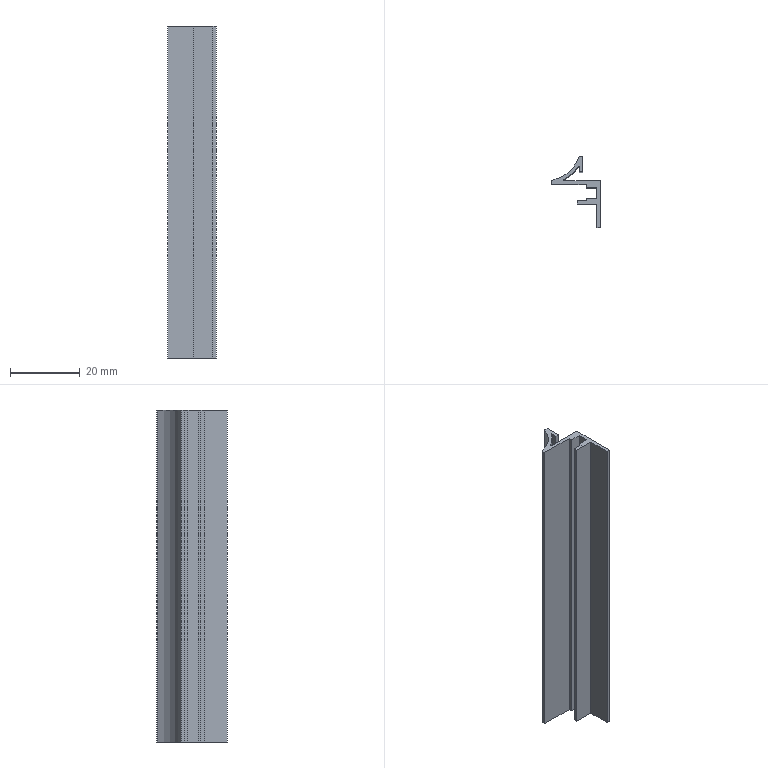Part | SolidWorks | features BaseBody 1, ICE 1, MoveFace 1 | 1 solid | 27 faces | box 14 x 20.3 x 95 mm | volume 4837 mm3 | plane 20 | cylinder 7 | commonest cylinder face diameters 0.387 x2 0.8 x2 0.4 x1 20 x1 22 x1
STEP:
#1=CARTESIAN_POINT('',(-5.304,-0.625,200.));
#2=VERTEX_POINT('',#1);
#3=CARTESIAN_POINT('',(-5.449,-0.8125,200.));
#4=VERTEX_POINT('',#3);
#5=CARTESIAN_POINT('',(-5.255,-0.8125,200.));
#6=DIRECTION('',(0.,0.,1.));
#7=DIRECTION('',(-1.,0.,0.));
#8=AXIS2_PLACEMENT_3D('',#5,#6,#7);
#9=CIRCLE('',#8,0.1937);
#10=EDGE_CURVE('',#2,#4,#9,.T.);
#11=ORIENTED_EDGE('',*,*,#10,.T.);
#12=CARTESIAN_POINT('',(-5.449,-0.8125,105.));
#13=VERTEX_POINT('',#12);
#14=CARTESIAN_POINT('',(-5.449,-0.8125,230.));
#15=DIRECTION('',(0.,0.,-1.));
#16=VECTOR('',#15,1000.);
#17=LINE('',#14,#16);
#18=EDGE_CURVE('',#4,#13,#17,.T.);
#19=ORIENTED_EDGE('',*,*,#18,.T.);
#20=CARTESIAN_POINT('',(-5.304,-0.625,105.));
#21=VERTEX_POINT('',#20);
#22=CARTESIAN_POINT('',(-5.255,-0.8125,105.));
#23=DIRECTION('',(0.,0.,-1.));
#24=DIRECTION('',(1.,0.,0.));
#25=AXIS2_PLACEMENT_3D('',#22,#23,#24);
#26=CIRCLE('',#25,0.1937);
#27=EDGE_CURVE('',#13,#21,#26,.T.);
#28=ORIENTED_EDGE('',*,*,#27,.T.);
#29=CARTESIAN_POINT('',(-5.304,-0.625,230.));
#30=DIRECTION('',(0.,0.,-1.));
#31=VECTOR('',#30,1000.);
#32=LINE('',#29,#31);
#33=EDGE_CURVE('',#2,#21,#32,.T.);
#34=ORIENTED_EDGE('',*,*,#33,.F.);
#35=EDGE_LOOP('',(#11,#19,#28,#34));
#36=FACE_OUTER_BOUND('',#35,.T.);
#37=CARTESIAN_POINT('',(-5.255,-0.8125,230.));
#38=DIRECTION('',(0.,0.,-1.));
#39=DIRECTION('',(-1.,0.,0.));
#40=AXIS2_PLACEMENT_3D('',#37,#38,#39);
#41=CYLINDRICAL_SURFACE('',#40,0.1937);
#42=ADVANCED_FACE('',(#36),#41,.F.);
#43=CARTESIAN_POINT('',(5.,-1.,105.));
#44=VERTEX_POINT('',#43);
#45=CARTESIAN_POINT('',(5.,-14.3,105.));
#46=VERTEX_POINT('',#45);
#47=CARTESIAN_POINT('',(5.,29.623,105.));
#48=DIRECTION('',(0.,-1.,0.));
#49=VECTOR('',#48,1000.);
#50=LINE('',#47,#49);
#51=EDGE_CURVE('',#44,#46,#50,.T.);
#52=ORIENTED_EDGE('',*,*,#51,.F.);
#53=CARTESIAN_POINT('',(5.,-1.,200.));
#54=VERTEX_POINT('',#53);
#55=CARTESIAN_POINT('',(5.,-1.,230.));
#56=DIRECTION('',(0.,0.,-1.));
#57=VECTOR('',#56,1000.);
#58=LINE('',#55,#57);
#59=EDGE_CURVE('',#54,#44,#58,.T.);
#60=ORIENTED_EDGE('',*,*,#59,.F.);
#61=CARTESIAN_POINT('',(5.,-14.3,200.));
#62=VERTEX_POINT('',#61);
#63=CARTESIAN_POINT('',(5.,-14.3,200.));
#64=DIRECTION('',(0.,1.,0.));
#65=VECTOR('',#64,1000.);
#66=LINE('',#63,#65);
#67=EDGE_CURVE('',#62,#54,#66,.T.);
#68=ORIENTED_EDGE('',*,*,#67,.F.);
#69=CARTESIAN_POINT('',(5.,-14.3,230.));
#70=DIRECTION('',(0.,0.,1.));
#71=VECTOR('',#70,1000.);
#72=LINE('',#69,#71);
#73=EDGE_CURVE('',#46,#62,#72,.T.);
#74=ORIENTED_EDGE('',*,*,#73,.F.);
#75=EDGE_LOOP('',(#52,#60,#68,#74));
#76=FACE_OUTER_BOUND('',#75,.T.);
#77=CARTESIAN_POINT('',(5.,-14.3,230.));
#78=DIRECTION('',(-1.,0.,0.));
#79=DIRECTION('',(0.,0.,1.));
#80=AXIS2_PLACEMENT_3D('',#77,#78,#79);
#81=PLANE('',#80);
#82=ADVANCED_FACE('',(#76),#81,.F.);
#83=CARTESIAN_POINT('',(-9.,-2.,105.));
#84=VERTEX_POINT('',#83);
#85=CARTESIAN_POINT('',(-9.,-2.,200.));
#86=VERTEX_POINT('',#85);
#87=CARTESIAN_POINT('',(-9.,-2.,230.));
#88=DIRECTION('',(0.,0.,1.));
#89=VECTOR('',#88,1000.);
#90=LINE('',#87,#89);
#91=EDGE_CURVE('',#84,#86,#90,.T.);
#92=ORIENTED_EDGE('',*,*,#91,.F.);
#93=CARTESIAN_POINT('',(0.9,-2.,105.));
#94=VERTEX_POINT('',#93);
#95=CARTESIAN_POINT('',(5.,-2.,105.));
#96=DIRECTION('',(-1.,0.,0.));
#97=VECTOR('',#96,1000.);
#98=LINE('',#95,#97);
#99=EDGE_CURVE('',#94,#84,#98,.T.);
#100=ORIENTED_EDGE('',*,*,#99,.F.);
#101=CARTESIAN_POINT('',(0.9,-2.,200.));
#102=VERTEX_POINT('',#101);
#103=CARTESIAN_POINT('',(0.9,-2.,230.));
#104=DIRECTION('',(0.,0.,-1.));
#105=VECTOR('',#104,1000.);
#106=LINE('',#103,#105);
#107=EDGE_CURVE('',#102,#94,#106,.T.);
#108=ORIENTED_EDGE('',*,*,#107,.F.);
#109=CARTESIAN_POINT('',(5.,-2.,200.));
#110=DIRECTION('',(1.,0.,0.));
#111=VECTOR('',#110,1000.);
#112=LINE('',#109,#111);
#113=EDGE_CURVE('',#86,#102,#112,.T.);
#114=ORIENTED_EDGE('',*,*,#113,.F.);
#115=EDGE_LOOP('',(#92,#100,#108,#114));
#116=FACE_OUTER_BOUND('',#115,.T.);
#117=CARTESIAN_POINT('',(-9.,-2.,230.));
#118=DIRECTION('',(0.,1.,0.));
#119=DIRECTION('',(0.,0.,1.));
#120=AXIS2_PLACEMENT_3D('',#117,#118,#119);
#121=PLANE('',#120);
#122=ADVANCED_FACE('',(#116),#121,.F.);
#123=CARTESIAN_POINT('',(4.,-6.,200.));
#124=VERTEX_POINT('',#123);
#125=CARTESIAN_POINT('',(4.,-3.,200.));
#126=VERTEX_POINT('',#125);
#127=CARTESIAN_POINT('',(4.,29.623,200.));
#128=DIRECTION('',(0.,1.,0.));
#129=VECTOR('',#128,1000.);
#130=LINE('',#127,#129);
#131=EDGE_CURVE('',#124,#126,#130,.T.);
#132=ORIENTED_EDGE('',*,*,#131,.F.);
#133=CARTESIAN_POINT('',(1.,-6.,200.));
#134=VERTEX_POINT('',#133);
#135=CARTESIAN_POINT('',(5.,-6.,200.));
#136=DIRECTION('',(1.,0.,0.));
#137=VECTOR('',#136,1000.);
#138=LINE('',#135,#137);
#139=EDGE_CURVE('',#134,#124,#138,.T.);
#140=ORIENTED_EDGE('',*,*,#139,.F.);
#141=CARTESIAN_POINT('',(1.,-6.7,200.));
#142=VERTEX_POINT('',#141);
#143=CARTESIAN_POINT('',(1.,-6.,200.));
#144=DIRECTION('',(0.,-1.,0.));
#145=VECTOR('',#144,1000.);
#146=LINE('',#143,#145);
#147=EDGE_CURVE('',#134,#142,#146,.T.);
#148=ORIENTED_EDGE('',*,*,#147,.T.);
#149=CARTESIAN_POINT('',(-1.7,-6.7,200.));
#150=VERTEX_POINT('',#149);
#151=CARTESIAN_POINT('',(5.,-6.7,200.));
#152=DIRECTION('',(1.,0.,0.));
#153=VECTOR('',#152,1000.);
#154=LINE('',#151,#153);
#155=EDGE_CURVE('',#150,#142,#154,.T.);
#156=ORIENTED_EDGE('',*,*,#155,.F.);
#157=CARTESIAN_POINT('',(-1.7,-7.7,200.));
#158=VERTEX_POINT('',#157);
#159=CARTESIAN_POINT('',(-1.7,-6.7,200.));
#160=DIRECTION('',(0.,-1.,0.));
#161=VECTOR('',#160,1000.);
#162=LINE('',#159,#161);
#163=EDGE_CURVE('',#150,#158,#162,.T.);
#164=ORIENTED_EDGE('',*,*,#163,.T.);
#165=CARTESIAN_POINT('',(4.,-7.7,200.));
#166=VERTEX_POINT('',#165);
#167=CARTESIAN_POINT('',(5.,-7.7,200.));
#168=DIRECTION('',(-1.,0.,0.));
#169=VECTOR('',#168,1000.);
#170=LINE('',#167,#169);
#171=EDGE_CURVE('',#166,#158,#170,.T.);
#172=ORIENTED_EDGE('',*,*,#171,.F.);
#173=CARTESIAN_POINT('',(4.,-14.3,200.));
#174=VERTEX_POINT('',#173);
#175=CARTESIAN_POINT('',(4.,29.623,200.));
#176=DIRECTION('',(0.,1.,0.));
#177=VECTOR('',#176,1000.);
#178=LINE('',#175,#177);
#179=EDGE_CURVE('',#174,#166,#178,.T.);
#180=ORIENTED_EDGE('',*,*,#179,.F.);
#181=CARTESIAN_POINT('',(5.,-14.3,200.));
#182=DIRECTION('',(-1.,0.,0.));
#183=VECTOR('',#182,1000.);
#184=LINE('',#181,#183);
#185=EDGE_CURVE('',#62,#174,#184,.T.);
#186=ORIENTED_EDGE('',*,*,#185,.F.);
#187=ORIENTED_EDGE('',*,*,#67,.T.);
#188=CARTESIAN_POINT('',(-5.207,-1.,200.));
#189=VERTEX_POINT('',#188);
#190=CARTESIAN_POINT('',(5.,-1.,200.));
#191=DIRECTION('',(1.,0.,0.));
#192=VECTOR('',#191,1000.);
#193=LINE('',#190,#192);
#194=EDGE_CURVE('',#189,#54,#193,.T.);
#195=ORIENTED_EDGE('',*,*,#194,.F.);
#196=CARTESIAN_POINT('',(-5.255,-0.8125,200.));
#197=DIRECTION('',(0.,0.,1.));
#198=DIRECTION('',(-1.,0.,0.));
#199=AXIS2_PLACEMENT_3D('',#196,#197,#198);
#200=CIRCLE('',#199,0.1937);
#201=EDGE_CURVE('',#4,#189,#200,.T.);
#202=ORIENTED_EDGE('',*,*,#201,.F.);
#203=ORIENTED_EDGE('',*,*,#10,.F.);
#204=CARTESIAN_POINT('',(-1.368,3.063,200.));
#205=VERTEX_POINT('',#204);
#206=CARTESIAN_POINT('',(-10.628,9.,200.));
#207=DIRECTION('',(0.,0.,1.));
#208=DIRECTION('',(-1.,0.,0.));
#209=AXIS2_PLACEMENT_3D('',#206,#207,#208);
#210=CIRCLE('',#209,11.);
#211=EDGE_CURVE('',#2,#205,#210,.T.);
#212=ORIENTED_EDGE('',*,*,#211,.T.);
#213=CARTESIAN_POINT('',(-1.,2.955,200.));
#214=VERTEX_POINT('',#213);
#215=CARTESIAN_POINT('',(-1.2,2.955,200.));
#216=DIRECTION('',(0.,0.,1.));
#217=DIRECTION('',(-1.,0.,0.));
#218=AXIS2_PLACEMENT_3D('',#215,#216,#217);
#219=CIRCLE('',#218,0.2);
#220=EDGE_CURVE('',#214,#205,#219,.T.);
#221=ORIENTED_EDGE('',*,*,#220,.F.);
#222=CARTESIAN_POINT('',(-1.,1.5,200.));
#223=VERTEX_POINT('',#222);
#224=CARTESIAN_POINT('',(-1.,2.955,200.));
#225=DIRECTION('',(0.,1.,0.));
#226=VECTOR('',#225,1000.);
#227=LINE('',#224,#226);
#228=EDGE_CURVE('',#223,#214,#227,.T.);
#229=ORIENTED_EDGE('',*,*,#228,.F.);
#230=CARTESIAN_POINT('',(0.,1.5,200.));
#231=VERTEX_POINT('',#230);
#232=CARTESIAN_POINT('',(-1.,1.5,200.));
#233=DIRECTION('',(-1.,0.,0.));
#234=VECTOR('',#233,1000.);
#235=LINE('',#232,#234);
#236=EDGE_CURVE('',#231,#223,#235,.T.);
#237=ORIENTED_EDGE('',*,*,#236,.F.);
#238=CARTESIAN_POINT('',(0.,6.,200.));
#239=VERTEX_POINT('',#238);
#240=CARTESIAN_POINT('',(0.,1.5,200.));
#241=DIRECTION('',(0.,-1.,0.));
#242=VECTOR('',#241,1000.);
#243=LINE('',#240,#242);
#244=EDGE_CURVE('',#239,#231,#243,.T.);
#245=ORIENTED_EDGE('',*,*,#244,.F.);
#246=CARTESIAN_POINT('',(-0.8,6.,200.));
#247=VERTEX_POINT('',#246);
#248=CARTESIAN_POINT('',(0.,6.,200.));
#249=DIRECTION('',(1.,0.,0.));
#250=VECTOR('',#249,1000.);
#251=LINE('',#248,#250);
#252=EDGE_CURVE('',#247,#239,#251,.T.);
#253=ORIENTED_EDGE('',*,*,#252,.F.);
#254=CARTESIAN_POINT('',(-1.178,5.731,200.));
#255=VERTEX_POINT('',#254);
#256=CARTESIAN_POINT('',(-0.8,5.6,200.));
#257=DIRECTION('',(0.,0.,1.));
#258=DIRECTION('',(-1.,0.,0.));
#259=AXIS2_PLACEMENT_3D('',#256,#257,#258);
#260=CIRCLE('',#259,0.4);
#261=EDGE_CURVE('',#247,#255,#260,.T.);
#262=ORIENTED_EDGE('',*,*,#261,.T.);
#263=CARTESIAN_POINT('',(-8.678,-0.8077,200.));
#264=VERTEX_POINT('',#263);
#265=CARTESIAN_POINT('',(-10.628,9.,200.));
#266=DIRECTION('',(0.,0.,1.));
#267=DIRECTION('',(-1.,0.,0.));
#268=AXIS2_PLACEMENT_3D('',#265,#266,#267);
#269=CIRCLE('',#268,10.);
#270=EDGE_CURVE('',#264,#255,#269,.T.);
#271=ORIENTED_EDGE('',*,*,#270,.F.);
#272=CARTESIAN_POINT('',(-9.,-1.2,200.));
#273=VERTEX_POINT('',#272);
#274=CARTESIAN_POINT('',(-8.6,-1.2,200.));
#275=DIRECTION('',(0.,0.,1.));
#276=DIRECTION('',(-1.,0.,0.));
#277=AXIS2_PLACEMENT_3D('',#274,#275,#276);
#278=CIRCLE('',#277,0.4);
#279=EDGE_CURVE('',#264,#273,#278,.T.);
#280=ORIENTED_EDGE('',*,*,#279,.T.);
#281=CARTESIAN_POINT('',(-9.,8.,200.));
#282=DIRECTION('',(0.,-1.,0.));
#283=VECTOR('',#282,1000.);
#284=LINE('',#281,#283);
#285=EDGE_CURVE('',#273,#86,#284,.T.);
#286=ORIENTED_EDGE('',*,*,#285,.T.);
#287=ORIENTED_EDGE('',*,*,#113,.T.);
#288=CARTESIAN_POINT('',(0.9,-3.,200.));
#289=VERTEX_POINT('',#288);
#290=CARTESIAN_POINT('',(0.9,29.623,200.));
#291=DIRECTION('',(0.,1.,0.));
#292=VECTOR('',#291,1000.);
#293=LINE('',#290,#292);
#294=EDGE_CURVE('',#289,#102,#293,.T.);
#295=ORIENTED_EDGE('',*,*,#294,.F.);
#296=CARTESIAN_POINT('',(5.,-3.,200.));
#297=DIRECTION('',(-1.,0.,0.));
#298=VECTOR('',#297,1000.);
#299=LINE('',#296,#298);
#300=EDGE_CURVE('',#126,#289,#299,.T.);
#301=ORIENTED_EDGE('',*,*,#300,.F.);
#302=EDGE_LOOP('',(#132,#140,#148,#156,#164,#172,#180,#186,#187,#195,#202,#203,#212,#221,#229,#237,#245,#253,#262,#271,#280,#286,#287,#295,#301));
#303=FACE_OUTER_BOUND('',#302,.T.);
#304=CARTESIAN_POINT('',(5.,29.623,200.));
#305=DIRECTION('',(0.,0.,-1.));
#306=DIRECTION('',(-1.,0.,0.));
#307=AXIS2_PLACEMENT_3D('',#304,#305,#306);
#308=PLANE('',#307);
#309=ADVANCED_FACE('',(#303),#308,.F.);
#310=ORIENTED_EDGE('',*,*,#185,.T.);
#311=CARTESIAN_POINT('',(4.,-14.3,105.));
#312=VERTEX_POINT('',#311);
#313=CARTESIAN_POINT('',(4.,-14.3,230.));
#314=DIRECTION('',(0.,0.,1.));
#315=VECTOR('',#314,1000.);
#316=LINE('',#313,#315);
#317=EDGE_CURVE('',#312,#174,#316,.T.);
#318=ORIENTED_EDGE('',*,*,#317,.F.);
#319=CARTESIAN_POINT('',(5.,-14.3,105.));
#320=DIRECTION('',(-1.,0.,0.));
#321=VECTOR('',#320,1000.);
#322=LINE('',#319,#321);
#323=EDGE_CURVE('',#46,#312,#322,.T.);
#324=ORIENTED_EDGE('',*,*,#323,.F.);
#325=ORIENTED_EDGE('',*,*,#73,.T.);
#326=EDGE_LOOP('',(#310,#318,#324,#325));
#327=FACE_OUTER_BOUND('',#326,.T.);
#328=CARTESIAN_POINT('',(4.,-14.3,230.));
#329=DIRECTION('',(0.,1.,0.));
#330=DIRECTION('',(0.,0.,1.));
#331=AXIS2_PLACEMENT_3D('',#328,#329,#330);
#332=PLANE('',#331);
#333=ADVANCED_FACE('',(#327),#332,.F.);
#334=ORIENTED_EDGE('',*,*,#51,.T.);
#335=ORIENTED_EDGE('',*,*,#323,.T.);
#336=CARTESIAN_POINT('',(4.,-7.7,105.));
#337=VERTEX_POINT('',#336);
#338=CARTESIAN_POINT('',(4.,-7.7,105.));
#339=DIRECTION('',(0.,-1.,0.));
#340=VECTOR('',#339,1000.);
#341=LINE('',#338,#340);
#342=EDGE_CURVE('',#337,#312,#341,.T.);
#343=ORIENTED_EDGE('',*,*,#342,.F.);
#344=CARTESIAN_POINT('',(-1.7,-7.7,105.));
#345=VERTEX_POINT('',#344);
#346=CARTESIAN_POINT('',(-1.7,-7.7,105.));
#347=DIRECTION('',(1.,0.,0.));
#348=VECTOR('',#347,1000.);
#349=LINE('',#346,#348);
#350=EDGE_CURVE('',#345,#337,#349,.T.);
#351=ORIENTED_EDGE('',*,*,#350,.F.);
#352=CARTESIAN_POINT('',(-1.7,-6.7,105.));
#353=VERTEX_POINT('',#352);
#354=CARTESIAN_POINT('',(-1.7,29.623,105.));
#355=DIRECTION('',(0.,1.,0.));
#356=VECTOR('',#355,1000.);
#357=LINE('',#354,#356);
#358=EDGE_CURVE('',#345,#353,#357,.T.);
#359=ORIENTED_EDGE('',*,*,#358,.T.);
#360=CARTESIAN_POINT('',(1.,-6.7,105.));
#361=VERTEX_POINT('',#360);
#362=CARTESIAN_POINT('',(1.,-6.7,105.));
#363=DIRECTION('',(-1.,0.,0.));
#364=VECTOR('',#363,1000.);
#365=LINE('',#362,#364);
#366=EDGE_CURVE('',#361,#353,#365,.T.);
#367=ORIENTED_EDGE('',*,*,#366,.F.);
#368=CARTESIAN_POINT('',(1.,-6.,105.));
#369=VERTEX_POINT('',#368);
#370=CARTESIAN_POINT('',(1.,29.623,105.));
#371=DIRECTION('',(0.,1.,0.));
#372=VECTOR('',#371,1000.);
#373=LINE('',#370,#372);
#374=EDGE_CURVE('',#361,#369,#373,.T.);
#375=ORIENTED_EDGE('',*,*,#374,.T.);
#376=CARTESIAN_POINT('',(4.,-6.,105.));
#377=VERTEX_POINT('',#376);
#378=CARTESIAN_POINT('',(4.,-6.,105.));
#379=DIRECTION('',(-1.,0.,0.));
#380=VECTOR('',#379,1000.);
#381=LINE('',#378,#380);
#382=EDGE_CURVE('',#377,#369,#381,.T.);
#383=ORIENTED_EDGE('',*,*,#382,.F.);
#384=CARTESIAN_POINT('',(4.,-3.,105.));
#385=VERTEX_POINT('',#384);
#386=CARTESIAN_POINT('',(4.,-3.,105.));
#387=DIRECTION('',(0.,-1.,0.));
#388=VECTOR('',#387,1000.);
#389=LINE('',#386,#388);
#390=EDGE_CURVE('',#385,#377,#389,.T.);
#391=ORIENTED_EDGE('',*,*,#390,.F.);
#392=CARTESIAN_POINT('',(0.9,-3.,105.));
#393=VERTEX_POINT('',#392);
#394=CARTESIAN_POINT('',(0.9,-3.,105.));
#395=DIRECTION('',(1.,0.,0.));
#396=VECTOR('',#395,1000.);
#397=LINE('',#394,#396);
#398=EDGE_CURVE('',#393,#385,#397,.T.);
#399=ORIENTED_EDGE('',*,*,#398,.F.);
#400=CARTESIAN_POINT('',(0.9,-2.,105.));
#401=DIRECTION('',(0.,-1.,0.));
#402=VECTOR('',#401,1000.);
#403=LINE('',#400,#402);
#404=EDGE_CURVE('',#94,#393,#403,.T.);
#405=ORIENTED_EDGE('',*,*,#404,.F.);
#406=ORIENTED_EDGE('',*,*,#99,.T.);
#407=CARTESIAN_POINT('',(-9.,-1.2,105.));
#408=VERTEX_POINT('',#407);
#409=CARTESIAN_POINT('',(-9.,-1.2,105.));
#410=DIRECTION('',(0.,-1.,0.));
#411=VECTOR('',#410,1000.);
#412=LINE('',#409,#411);
#413=EDGE_CURVE('',#408,#84,#412,.T.);
#414=ORIENTED_EDGE('',*,*,#413,.F.);
#415=CARTESIAN_POINT('',(-8.678,-0.8077,105.));
#416=VERTEX_POINT('',#415);
#417=CARTESIAN_POINT('',(-8.6,-1.2,105.));
#418=DIRECTION('',(0.,0.,-1.));
#419=DIRECTION('',(1.,0.,0.));
#420=AXIS2_PLACEMENT_3D('',#417,#418,#419);
#421=CIRCLE('',#420,0.4);
#422=EDGE_CURVE('',#408,#416,#421,.T.);
#423=ORIENTED_EDGE('',*,*,#422,.T.);
#424=CARTESIAN_POINT('',(-1.178,5.731,105.));
#425=VERTEX_POINT('',#424);
#426=CARTESIAN_POINT('',(-10.628,9.,105.));
#427=DIRECTION('',(0.,0.,-1.));
#428=DIRECTION('',(1.,0.,0.));
#429=AXIS2_PLACEMENT_3D('',#426,#427,#428);
#430=CIRCLE('',#429,10.);
#431=EDGE_CURVE('',#425,#416,#430,.T.);
#432=ORIENTED_EDGE('',*,*,#431,.F.);
#433=CARTESIAN_POINT('',(-0.8,6.,105.));
#434=VERTEX_POINT('',#433);
#435=CARTESIAN_POINT('',(-0.8,5.6,105.));
#436=DIRECTION('',(0.,0.,-1.));
#437=DIRECTION('',(1.,0.,0.));
#438=AXIS2_PLACEMENT_3D('',#435,#436,#437);
#439=CIRCLE('',#438,0.4);
#440=EDGE_CURVE('',#425,#434,#439,.T.);
#441=ORIENTED_EDGE('',*,*,#440,.T.);
#442=CARTESIAN_POINT('',(0.,6.,105.));
#443=VERTEX_POINT('',#442);
#444=CARTESIAN_POINT('',(0.,6.,105.));
#445=DIRECTION('',(-1.,0.,0.));
#446=VECTOR('',#445,1000.);
#447=LINE('',#444,#446);
#448=EDGE_CURVE('',#443,#434,#447,.T.);
#449=ORIENTED_EDGE('',*,*,#448,.F.);
#450=CARTESIAN_POINT('',(0.,1.5,105.));
#451=VERTEX_POINT('',#450);
#452=CARTESIAN_POINT('',(0.,1.5,105.));
#453=DIRECTION('',(0.,1.,0.));
#454=VECTOR('',#453,1000.);
#455=LINE('',#452,#454);
#456=EDGE_CURVE('',#451,#443,#455,.T.);
#457=ORIENTED_EDGE('',*,*,#456,.F.);
#458=CARTESIAN_POINT('',(-1.,1.5,105.));
#459=VERTEX_POINT('',#458);
#460=CARTESIAN_POINT('',(-1.,1.5,105.));
#461=DIRECTION('',(1.,0.,0.));
#462=VECTOR('',#461,1000.);
#463=LINE('',#460,#462);
#464=EDGE_CURVE('',#459,#451,#463,.T.);
#465=ORIENTED_EDGE('',*,*,#464,.F.);
#466=CARTESIAN_POINT('',(-1.,2.955,105.));
#467=VERTEX_POINT('',#466);
#468=CARTESIAN_POINT('',(-1.,2.955,105.));
#469=DIRECTION('',(0.,-1.,0.));
#470=VECTOR('',#469,1000.);
#471=LINE('',#468,#470);
#472=EDGE_CURVE('',#467,#459,#471,.T.);
#473=ORIENTED_EDGE('',*,*,#472,.F.);
#474=CARTESIAN_POINT('',(-1.368,3.063,105.));
#475=VERTEX_POINT('',#474);
#476=CARTESIAN_POINT('',(-1.2,2.955,105.));
#477=DIRECTION('',(0.,0.,-1.));
#478=DIRECTION('',(1.,0.,0.));
#479=AXIS2_PLACEMENT_3D('',#476,#477,#478);
#480=CIRCLE('',#479,0.2);
#481=EDGE_CURVE('',#475,#467,#480,.T.);
#482=ORIENTED_EDGE('',*,*,#481,.F.);
#483=CARTESIAN_POINT('',(-10.628,9.,105.));
#484=DIRECTION('',(0.,0.,-1.));
#485=DIRECTION('',(1.,0.,0.));
#486=AXIS2_PLACEMENT_3D('',#483,#484,#485);
#487=CIRCLE('',#486,11.);
#488=EDGE_CURVE('',#475,#21,#487,.T.);
#489=ORIENTED_EDGE('',*,*,#488,.T.);
#490=ORIENTED_EDGE('',*,*,#27,.F.);
#491=CARTESIAN_POINT('',(-5.207,-1.,105.));
#492=VERTEX_POINT('',#491);
#493=CARTESIAN_POINT('',(-5.255,-0.8125,105.));
#494=DIRECTION('',(0.,0.,-1.));
#495=DIRECTION('',(1.,0.,0.));
#496=AXIS2_PLACEMENT_3D('',#493,#494,#495);
#497=CIRCLE('',#496,0.1937);
#498=EDGE_CURVE('',#492,#13,#497,.T.);
#499=ORIENTED_EDGE('',*,*,#498,.F.);
#500=CARTESIAN_POINT('',(5.,-1.,105.));
#501=DIRECTION('',(-1.,0.,0.));
#502=VECTOR('',#501,1000.);
#503=LINE('',#500,#502);
#504=EDGE_CURVE('',#44,#492,#503,.T.);
#505=ORIENTED_EDGE('',*,*,#504,.F.);
#506=EDGE_LOOP('',(#334,#335,#343,#351,#359,#367,#375,#383,#391,#399,#405,#406,#414,#423,#432,#441,#449,#457,#465,#473,#482,#489,#490,#499,#505));
#507=FACE_OUTER_BOUND('',#506,.T.);
#508=CARTESIAN_POINT('',(5.,29.623,105.));
#509=DIRECTION('',(0.,0.,1.));
#510=DIRECTION('',(1.,0.,0.));
#511=AXIS2_PLACEMENT_3D('',#508,#509,#510);
#512=PLANE('',#511);
#513=ADVANCED_FACE('',(#507),#512,.F.);
#514=ORIENTED_EDGE('',*,*,#59,.T.);
#515=ORIENTED_EDGE('',*,*,#504,.T.);
#516=CARTESIAN_POINT('',(-5.207,-1.,230.));
#517=DIRECTION('',(0.,0.,-1.));
#518=VECTOR('',#517,1000.);
#519=LINE('',#516,#518);
#520=EDGE_CURVE('',#189,#492,#519,.T.);
#521=ORIENTED_EDGE('',*,*,#520,.F.);
#522=ORIENTED_EDGE('',*,*,#194,.T.);
#523=EDGE_LOOP('',(#514,#515,#521,#522));
#524=FACE_OUTER_BOUND('',#523,.T.);
#525=CARTESIAN_POINT('',(5.,-1.,230.));
#526=DIRECTION('',(0.,-1.,0.));
#527=DIRECTION('',(0.,0.,-1.));
#528=AXIS2_PLACEMENT_3D('',#525,#526,#527);
#529=PLANE('',#528);
#530=ADVANCED_FACE('',(#524),#529,.F.);
#531=CARTESIAN_POINT('',(-9.,-1.2,230.));
#532=DIRECTION('',(0.,0.,1.));
#533=VECTOR('',#532,1000.);
#534=LINE('',#531,#533);
#535=EDGE_CURVE('',#408,#273,#534,.T.);
#536=ORIENTED_EDGE('',*,*,#535,.F.);
#537=ORIENTED_EDGE('',*,*,#413,.T.);
#538=ORIENTED_EDGE('',*,*,#91,.T.);
#539=ORIENTED_EDGE('',*,*,#285,.F.);
#540=EDGE_LOOP('',(#536,#537,#538,#539));
#541=FACE_OUTER_BOUND('',#540,.T.);
#542=CARTESIAN_POINT('',(-9.,-1.2,230.));
#543=DIRECTION('',(1.,0.,0.));
#544=DIRECTION('',(0.,0.,-1.));
#545=AXIS2_PLACEMENT_3D('',#542,#543,#544);
#546=PLANE('',#545);
#547=ADVANCED_FACE('',(#541),#546,.F.);
#548=ORIENTED_EDGE('',*,*,#294,.T.);
#549=ORIENTED_EDGE('',*,*,#107,.T.);
#550=ORIENTED_EDGE('',*,*,#404,.T.);
#551=CARTESIAN_POINT('',(0.9,-3.,230.));
#552=DIRECTION('',(0.,0.,-1.));
#553=VECTOR('',#552,1000.);
#554=LINE('',#551,#553);
#555=EDGE_CURVE('',#289,#393,#554,.T.);
#556=ORIENTED_EDGE('',*,*,#555,.F.);
#557=EDGE_LOOP('',(#548,#549,#550,#556));
#558=FACE_OUTER_BOUND('',#557,.T.);
#559=CARTESIAN_POINT('',(0.9,-2.,230.));
#560=DIRECTION('',(1.,0.,0.));
#561=DIRECTION('',(0.,0.,-1.));
#562=AXIS2_PLACEMENT_3D('',#559,#560,#561);
#563=PLANE('',#562);
#564=ADVANCED_FACE('',(#558),#563,.F.);
#565=ORIENTED_EDGE('',*,*,#300,.T.);
#566=ORIENTED_EDGE('',*,*,#555,.T.);
#567=ORIENTED_EDGE('',*,*,#398,.T.);
#568=CARTESIAN_POINT('',(4.,-3.,230.));
#569=DIRECTION('',(0.,0.,-1.));
#570=VECTOR('',#569,1000.);
#571=LINE('',#568,#570);
#572=EDGE_CURVE('',#126,#385,#571,.T.);
#573=ORIENTED_EDGE('',*,*,#572,.F.);
#574=EDGE_LOOP('',(#565,#566,#567,#573));
#575=FACE_OUTER_BOUND('',#574,.T.);
#576=CARTESIAN_POINT('',(0.9,-3.,230.));
#577=DIRECTION('',(0.,1.,0.));
#578=DIRECTION('',(0.,0.,1.));
#579=AXIS2_PLACEMENT_3D('',#576,#577,#578);
#580=PLANE('',#579);
#581=ADVANCED_FACE('',(#575),#580,.F.);
#582=ORIENTED_EDGE('',*,*,#131,.T.);
#583=ORIENTED_EDGE('',*,*,#572,.T.);
#584=ORIENTED_EDGE('',*,*,#390,.T.);
#585=CARTESIAN_POINT('',(4.,-6.,230.));
#586=DIRECTION('',(0.,0.,-1.));
#587=VECTOR('',#586,1000.);
#588=LINE('',#585,#587);
#589=EDGE_CURVE('',#124,#377,#588,.T.);
#590=ORIENTED_EDGE('',*,*,#589,.F.);
#591=EDGE_LOOP('',(#582,#583,#584,#590));
#592=FACE_OUTER_BOUND('',#591,.T.);
#593=CARTESIAN_POINT('',(4.,-3.,230.));
#594=DIRECTION('',(1.,0.,0.));
#595=DIRECTION('',(0.,0.,-1.));
#596=AXIS2_PLACEMENT_3D('',#593,#594,#595);
#597=PLANE('',#596);
#598=ADVANCED_FACE('',(#592),#597,.F.);
#599=ORIENTED_EDGE('',*,*,#139,.T.);
#600=ORIENTED_EDGE('',*,*,#589,.T.);
#601=ORIENTED_EDGE('',*,*,#382,.T.);
#602=CARTESIAN_POINT('',(1.,-6.,230.));
#603=DIRECTION('',(0.,0.,-1.));
#604=VECTOR('',#603,1000.);
#605=LINE('',#602,#604);
#606=EDGE_CURVE('',#134,#369,#605,.T.);
#607=ORIENTED_EDGE('',*,*,#606,.F.);
#608=EDGE_LOOP('',(#599,#600,#601,#607));
#609=FACE_OUTER_BOUND('',#608,.T.);
#610=CARTESIAN_POINT('',(4.,-6.,230.));
#611=DIRECTION('',(0.,-1.,0.));
#612=DIRECTION('',(0.,0.,-1.));
#613=AXIS2_PLACEMENT_3D('',#610,#611,#612);
#614=PLANE('',#613);
#615=ADVANCED_FACE('',(#609),#614,.F.);
#616=ORIENTED_EDGE('',*,*,#155,.T.);
#617=CARTESIAN_POINT('',(1.,-6.7,230.));
#618=DIRECTION('',(0.,0.,1.));
#619=VECTOR('',#618,1000.);
#620=LINE('',#617,#619);
#621=EDGE_CURVE('',#361,#142,#620,.T.);
#622=ORIENTED_EDGE('',*,*,#621,.F.);
#623=ORIENTED_EDGE('',*,*,#366,.T.);
#624=CARTESIAN_POINT('',(-1.7,-6.7,230.));
#625=DIRECTION('',(0.,0.,-1.));
#626=VECTOR('',#625,1000.);
#627=LINE('',#624,#626);
#628=EDGE_CURVE('',#150,#353,#627,.T.);
#629=ORIENTED_EDGE('',*,*,#628,.F.);
#630=EDGE_LOOP('',(#616,#622,#623,#629));
#631=FACE_OUTER_BOUND('',#630,.T.);
#632=CARTESIAN_POINT('',(1.,-6.7,230.));
#633=DIRECTION('',(0.,-1.,0.));
#634=DIRECTION('',(0.,0.,-1.));
#635=AXIS2_PLACEMENT_3D('',#632,#633,#634);
#636=PLANE('',#635);
#637=ADVANCED_FACE('',(#631),#636,.F.);
#638=ORIENTED_EDGE('',*,*,#171,.T.);
#639=CARTESIAN_POINT('',(-1.7,-7.7,230.));
#640=DIRECTION('',(0.,0.,1.));
#641=VECTOR('',#640,1000.);
#642=LINE('',#639,#641);
#643=EDGE_CURVE('',#345,#158,#642,.T.);
#644=ORIENTED_EDGE('',*,*,#643,.F.);
#645=ORIENTED_EDGE('',*,*,#350,.T.);
#646=CARTESIAN_POINT('',(4.,-7.7,230.));
#647=DIRECTION('',(0.,0.,-1.));
#648=VECTOR('',#647,1000.);
#649=LINE('',#646,#648);
#650=EDGE_CURVE('',#166,#337,#649,.T.);
#651=ORIENTED_EDGE('',*,*,#650,.F.);
#652=EDGE_LOOP('',(#638,#644,#645,#651));
#653=FACE_OUTER_BOUND('',#652,.T.);
#654=CARTESIAN_POINT('',(-1.7,-7.7,230.));
#655=DIRECTION('',(0.,1.,0.));
#656=DIRECTION('',(0.,0.,1.));
#657=AXIS2_PLACEMENT_3D('',#654,#655,#656);
#658=PLANE('',#657);
#659=ADVANCED_FACE('',(#653),#658,.F.);
#660=ORIENTED_EDGE('',*,*,#179,.T.);
#661=ORIENTED_EDGE('',*,*,#650,.T.);
#662=ORIENTED_EDGE('',*,*,#342,.T.);
#663=ORIENTED_EDGE('',*,*,#317,.T.);
#664=EDGE_LOOP('',(#660,#661,#662,#663));
#665=FACE_OUTER_BOUND('',#664,.T.);
#666=CARTESIAN_POINT('',(4.,-7.7,230.));
#667=DIRECTION('',(1.,0.,0.));
#668=DIRECTION('',(0.,0.,-1.));
#669=AXIS2_PLACEMENT_3D('',#666,#667,#668);
#670=PLANE('',#669);
#671=ADVANCED_FACE('',(#665),#670,.F.);
#672=ORIENTED_EDGE('',*,*,#18,.F.);
#673=ORIENTED_EDGE('',*,*,#201,.T.);
#674=ORIENTED_EDGE('',*,*,#520,.T.);
#675=ORIENTED_EDGE('',*,*,#498,.T.);
#676=EDGE_LOOP('',(#672,#673,#674,#675));
#677=FACE_OUTER_BOUND('',#676,.T.);
#678=CARTESIAN_POINT('',(-5.255,-0.8125,230.));
#679=DIRECTION('',(0.,0.,-1.));
#680=DIRECTION('',(-1.,0.,0.));
#681=AXIS2_PLACEMENT_3D('',#678,#679,#680);
#682=CYLINDRICAL_SURFACE('',#681,0.1937);
#683=ADVANCED_FACE('',(#677),#682,.F.);
#684=CARTESIAN_POINT('',(-1.,2.955,230.));
#685=DIRECTION('',(0.,0.,1.));
#686=VECTOR('',#685,1000.);
#687=LINE('',#684,#686);
#688=EDGE_CURVE('',#467,#214,#687,.T.);
#689=ORIENTED_EDGE('',*,*,#688,.F.);
#690=ORIENTED_EDGE('',*,*,#472,.T.);
#691=CARTESIAN_POINT('',(-1.,1.5,230.));
#692=DIRECTION('',(0.,0.,-1.));
#693=VECTOR('',#692,1000.);
#694=LINE('',#691,#693);
#695=EDGE_CURVE('',#223,#459,#694,.T.);
#696=ORIENTED_EDGE('',*,*,#695,.F.);
#697=ORIENTED_EDGE('',*,*,#228,.T.);
#698=EDGE_LOOP('',(#689,#690,#696,#697));
#699=FACE_OUTER_BOUND('',#698,.T.);
#700=CARTESIAN_POINT('',(-1.,2.955,230.));
#701=DIRECTION('',(1.,0.,0.));
#702=DIRECTION('',(0.,0.,-1.));
#703=AXIS2_PLACEMENT_3D('',#700,#701,#702);
#704=PLANE('',#703);
#705=ADVANCED_FACE('',(#699),#704,.F.);
#706=ORIENTED_EDGE('',*,*,#488,.F.);
#707=CARTESIAN_POINT('',(-1.368,3.063,230.));
#708=DIRECTION('',(0.,0.,1.));
#709=VECTOR('',#708,1000.);
#710=LINE('',#707,#709);
#711=EDGE_CURVE('',#475,#205,#710,.T.);
#712=ORIENTED_EDGE('',*,*,#711,.T.);
#713=ORIENTED_EDGE('',*,*,#211,.F.);
#714=ORIENTED_EDGE('',*,*,#33,.T.);
#715=EDGE_LOOP('',(#706,#712,#713,#714));
#716=FACE_OUTER_BOUND('',#715,.T.);
#717=CARTESIAN_POINT('',(-10.628,9.,230.));
#718=DIRECTION('',(0.,0.,-1.));
#719=DIRECTION('',(-1.,0.,0.));
#720=AXIS2_PLACEMENT_3D('',#717,#718,#719);
#721=CYLINDRICAL_SURFACE('',#720,11.);
#722=ADVANCED_FACE('',(#716),#721,.T.);
#723=CARTESIAN_POINT('',(-1.178,5.731,230.));
#724=DIRECTION('',(0.,0.,1.));
#725=VECTOR('',#724,1000.);
#726=LINE('',#723,#725);
#727=EDGE_CURVE('',#425,#255,#726,.T.);
#728=ORIENTED_EDGE('',*,*,#727,.F.);
#729=ORIENTED_EDGE('',*,*,#431,.T.);
#730=CARTESIAN_POINT('',(-8.678,-0.8077,230.));
#731=DIRECTION('',(0.,0.,-1.));
#732=VECTOR('',#731,1000.);
#733=LINE('',#730,#732);
#734=EDGE_CURVE('',#264,#416,#733,.T.);
#735=ORIENTED_EDGE('',*,*,#734,.F.);
#736=ORIENTED_EDGE('',*,*,#270,.T.);
#737=EDGE_LOOP('',(#728,#729,#735,#736));
#738=FACE_OUTER_BOUND('',#737,.T.);
#739=CARTESIAN_POINT('',(-10.628,9.,230.));
#740=DIRECTION('',(0.,0.,-1.));
#741=DIRECTION('',(-1.,0.,0.));
#742=AXIS2_PLACEMENT_3D('',#739,#740,#741);
#743=CYLINDRICAL_SURFACE('',#742,10.);
#744=ADVANCED_FACE('',(#738),#743,.F.);
#745=CARTESIAN_POINT('',(0.,1.5,230.));
#746=DIRECTION('',(0.,0.,1.));
#747=VECTOR('',#746,1000.);
#748=LINE('',#745,#747);
#749=EDGE_CURVE('',#451,#231,#748,.T.);
#750=ORIENTED_EDGE('',*,*,#749,.F.);
#751=ORIENTED_EDGE('',*,*,#456,.T.);
#752=CARTESIAN_POINT('',(0.,6.,230.));
#753=DIRECTION('',(0.,0.,-1.));
#754=VECTOR('',#753,1000.);
#755=LINE('',#752,#754);
#756=EDGE_CURVE('',#239,#443,#755,.T.);
#757=ORIENTED_EDGE('',*,*,#756,.F.);
#758=ORIENTED_EDGE('',*,*,#244,.T.);
#759=EDGE_LOOP('',(#750,#751,#757,#758));
#760=FACE_OUTER_BOUND('',#759,.T.);
#761=CARTESIAN_POINT('',(0.,1.5,230.));
#762=DIRECTION('',(-1.,0.,0.));
#763=DIRECTION('',(0.,0.,1.));
#764=AXIS2_PLACEMENT_3D('',#761,#762,#763);
#765=PLANE('',#764);
#766=ADVANCED_FACE('',(#760),#765,.F.);
#767=ORIENTED_EDGE('',*,*,#422,.F.);
#768=ORIENTED_EDGE('',*,*,#535,.T.);
#769=ORIENTED_EDGE('',*,*,#279,.F.);
#770=ORIENTED_EDGE('',*,*,#734,.T.);
#771=EDGE_LOOP('',(#767,#768,#769,#770));
#772=FACE_OUTER_BOUND('',#771,.T.);
#773=CARTESIAN_POINT('',(-8.6,-1.2,230.));
#774=DIRECTION('',(0.,0.,-1.));
#775=DIRECTION('',(-1.,0.,0.));
#776=AXIS2_PLACEMENT_3D('',#773,#774,#775);
#777=CYLINDRICAL_SURFACE('',#776,0.4);
#778=ADVANCED_FACE('',(#772),#777,.T.);
#779=ORIENTED_EDGE('',*,*,#147,.F.);
#780=ORIENTED_EDGE('',*,*,#606,.T.);
#781=ORIENTED_EDGE('',*,*,#374,.F.);
#782=ORIENTED_EDGE('',*,*,#621,.T.);
#783=EDGE_LOOP('',(#779,#780,#781,#782));
#784=FACE_OUTER_BOUND('',#783,.T.);
#785=CARTESIAN_POINT('',(1.,-6.,230.));
#786=DIRECTION('',(1.,0.,0.));
#787=DIRECTION('',(0.,0.,-1.));
#788=AXIS2_PLACEMENT_3D('',#785,#786,#787);
#789=PLANE('',#788);
#790=ADVANCED_FACE('',(#784),#789,.F.);
#791=ORIENTED_EDGE('',*,*,#163,.F.);
#792=ORIENTED_EDGE('',*,*,#628,.T.);
#793=ORIENTED_EDGE('',*,*,#358,.F.);
#794=ORIENTED_EDGE('',*,*,#643,.T.);
#795=EDGE_LOOP('',(#791,#792,#793,#794));
#796=FACE_OUTER_BOUND('',#795,.T.);
#797=CARTESIAN_POINT('',(-1.7,-6.7,230.));
#798=DIRECTION('',(1.,0.,0.));
#799=DIRECTION('',(0.,0.,-1.));
#800=AXIS2_PLACEMENT_3D('',#797,#798,#799);
#801=PLANE('',#800);
#802=ADVANCED_FACE('',(#796),#801,.F.);
#803=ORIENTED_EDGE('',*,*,#711,.F.);
#804=ORIENTED_EDGE('',*,*,#481,.T.);
#805=ORIENTED_EDGE('',*,*,#688,.T.);
#806=ORIENTED_EDGE('',*,*,#220,.T.);
#807=EDGE_LOOP('',(#803,#804,#805,#806));
#808=FACE_OUTER_BOUND('',#807,.T.);
#809=CARTESIAN_POINT('',(-1.2,2.955,230.));
#810=DIRECTION('',(0.,0.,-1.));
#811=DIRECTION('',(-1.,0.,0.));
#812=AXIS2_PLACEMENT_3D('',#809,#810,#811);
#813=CYLINDRICAL_SURFACE('',#812,0.2);
#814=ADVANCED_FACE('',(#808),#813,.F.);
#815=ORIENTED_EDGE('',*,*,#695,.T.);
#816=ORIENTED_EDGE('',*,*,#464,.T.);
#817=ORIENTED_EDGE('',*,*,#749,.T.);
#818=ORIENTED_EDGE('',*,*,#236,.T.);
#819=EDGE_LOOP('',(#815,#816,#817,#818));
#820=FACE_OUTER_BOUND('',#819,.T.);
#821=CARTESIAN_POINT('',(-1.,1.5,230.));
#822=DIRECTION('',(0.,1.,0.));
#823=DIRECTION('',(0.,0.,1.));
#824=AXIS2_PLACEMENT_3D('',#821,#822,#823);
#825=PLANE('',#824);
#826=ADVANCED_FACE('',(#820),#825,.F.);
#827=ORIENTED_EDGE('',*,*,#440,.F.);
#828=ORIENTED_EDGE('',*,*,#727,.T.);
#829=ORIENTED_EDGE('',*,*,#261,.F.);
#830=CARTESIAN_POINT('',(-0.8,6.,230.));
#831=DIRECTION('',(0.,0.,-1.));
#832=VECTOR('',#831,1000.);
#833=LINE('',#830,#832);
#834=EDGE_CURVE('',#247,#434,#833,.T.);
#835=ORIENTED_EDGE('',*,*,#834,.T.);
#836=EDGE_LOOP('',(#827,#828,#829,#835));
#837=FACE_OUTER_BOUND('',#836,.T.);
#838=CARTESIAN_POINT('',(-0.8,5.6,230.));
#839=DIRECTION('',(0.,0.,-1.));
#840=DIRECTION('',(-1.,0.,0.));
#841=AXIS2_PLACEMENT_3D('',#838,#839,#840);
#842=CYLINDRICAL_SURFACE('',#841,0.4);
#843=ADVANCED_FACE('',(#837),#842,.T.);
#844=ORIENTED_EDGE('',*,*,#756,.T.);
#845=ORIENTED_EDGE('',*,*,#448,.T.);
#846=ORIENTED_EDGE('',*,*,#834,.F.);
#847=ORIENTED_EDGE('',*,*,#252,.T.);
#848=EDGE_LOOP('',(#844,#845,#846,#847));
#849=FACE_OUTER_BOUND('',#848,.T.);
#850=CARTESIAN_POINT('',(0.,6.,230.));
#851=DIRECTION('',(0.,-1.,0.));
#852=DIRECTION('',(0.,0.,-1.));
#853=AXIS2_PLACEMENT_3D('',#850,#851,#852);
#854=PLANE('',#853);
#855=ADVANCED_FACE('',(#849),#854,.F.);
#856=CLOSED_SHELL('',(#42,#82,#122,#309,#333,#513,#530,#547,#564,#581,#598,#615,#637,#659,#671,#683,#705,#722,#744,#766,#778,#790,#802,#814,#826,#843,#855));
#857=MANIFOLD_SOLID_BREP('',#856);
#858=CARTESIAN_POINT('',(0.,0.,0.));
#859=DIRECTION('',(0.,0.,1.));
#860=DIRECTION('',(1.,0.,0.));
#861=AXIS2_PLACEMENT_3D('',#858,#859,#860);
#862=(LENGTH_UNIT()NAMED_UNIT(*)SI_UNIT(.MILLI.,.METRE.));
#863=UNCERTAINTY_MEASURE_WITH_UNIT(LENGTH_MEASURE(0.00001),#862,'','');
#864=(NAMED_UNIT(*)PLANE_ANGLE_UNIT()SI_UNIT($,.RADIAN.));
#865=(NAMED_UNIT(*)SI_UNIT($,.STERADIAN.)SOLID_ANGLE_UNIT());
#866=(GEOMETRIC_REPRESENTATION_CONTEXT(3)GLOBAL_UNCERTAINTY_ASSIGNED_CONTEXT((#863))GLOBAL_UNIT_ASSIGNED_CONTEXT((#862,#864,#865))REPRESENTATION_CONTEXT('',''));
#867=ADVANCED_BREP_SHAPE_REPRESENTATION('',(#857,#861),#866);